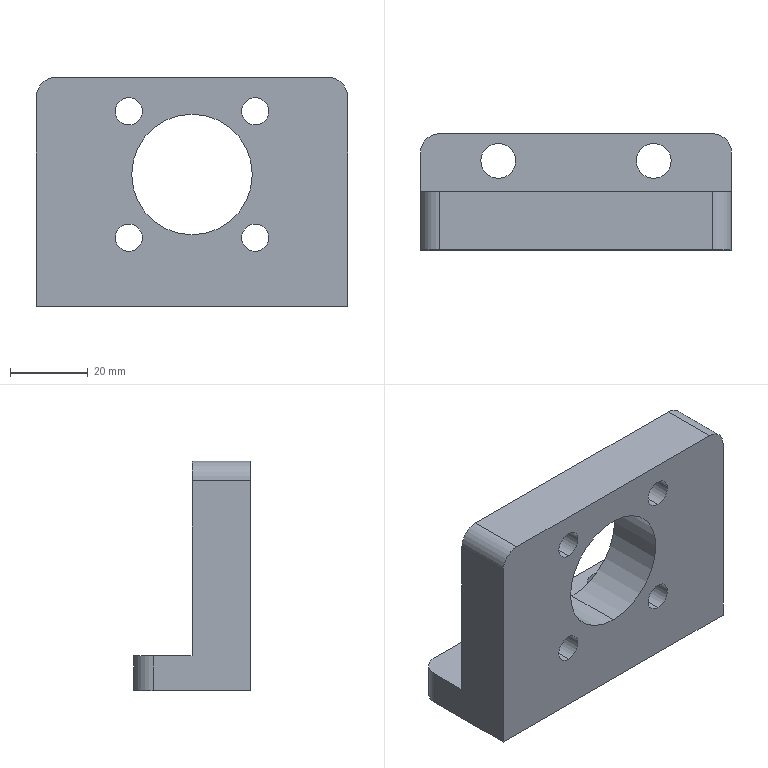Part | 1 solid | 38 faces | box 80 x 30 x 59 mm | volume 65210 mm3 | cylinder 26 | plane 12 | commonest cylinder face diameters 7 x8 11 x8 9 x4 10 x4 31 x2
STEP:
#1=CARTESIAN_POINT('',(16.263,-6.,44.763));
#2=VERTEX_POINT('',#1);
#3=CARTESIAN_POINT('',(16.263,-6.,55.763));
#4=VERTEX_POINT('',#3);
#5=CARTESIAN_POINT('',(16.263,-6.,50.263));
#6=DIRECTION('',(0.,1.,0.));
#7=DIRECTION('',(0.,0.,1.));
#8=AXIS2_PLACEMENT_3D('',#5,#6,#7);
#9=CIRCLE('',#8,5.5);
#10=EDGE_CURVE('',#2,#4,#9,.T.);
#11=ORIENTED_EDGE('',*,*,#10,.F.);
#12=CARTESIAN_POINT('',(16.263,0.,44.763));
#13=VERTEX_POINT('',#12);
#14=CARTESIAN_POINT('',(16.263,0.,44.763));
#15=DIRECTION('',(0.,1.,0.));
#16=VECTOR('',#15,1000.);
#17=LINE('',#14,#16);
#18=EDGE_CURVE('',#2,#13,#17,.T.);
#19=ORIENTED_EDGE('',*,*,#18,.T.);
#20=CARTESIAN_POINT('',(16.263,0.,55.763));
#21=VERTEX_POINT('',#20);
#22=CARTESIAN_POINT('',(16.263,0.,50.263));
#23=DIRECTION('',(0.,1.,0.));
#24=DIRECTION('',(0.,0.,1.));
#25=AXIS2_PLACEMENT_3D('',#22,#23,#24);
#26=CIRCLE('',#25,5.5);
#27=EDGE_CURVE('',#13,#21,#26,.T.);
#28=ORIENTED_EDGE('',*,*,#27,.T.);
#29=CARTESIAN_POINT('',(16.263,0.,55.763));
#30=DIRECTION('',(0.,1.,0.));
#31=VECTOR('',#30,1000.);
#32=LINE('',#29,#31);
#33=EDGE_CURVE('',#4,#21,#32,.T.);
#34=ORIENTED_EDGE('',*,*,#33,.F.);
#35=EDGE_LOOP('',(#11,#19,#28,#34));
#36=FACE_OUTER_BOUND('',#35,.T.);
#37=CARTESIAN_POINT('',(16.263,0.,50.263));
#38=DIRECTION('',(0.,1.,0.));
#39=DIRECTION('',(0.,0.,1.));
#40=AXIS2_PLACEMENT_3D('',#37,#38,#39);
#41=CYLINDRICAL_SURFACE('',#40,5.5);
#42=ADVANCED_FACE('',(#36),#41,.F.);
#43=CARTESIAN_POINT('',(16.263,-15.,46.763));
#44=VERTEX_POINT('',#43);
#45=CARTESIAN_POINT('',(16.263,-15.,53.763));
#46=VERTEX_POINT('',#45);
#47=CARTESIAN_POINT('',(16.263,-15.,50.263));
#48=DIRECTION('',(0.,1.,0.));
#49=DIRECTION('',(0.,0.,1.));
#50=AXIS2_PLACEMENT_3D('',#47,#48,#49);
#51=CIRCLE('',#50,3.5);
#52=EDGE_CURVE('',#44,#46,#51,.T.);
#53=ORIENTED_EDGE('',*,*,#52,.F.);
#54=CARTESIAN_POINT('',(16.263,-6.,46.763));
#55=VERTEX_POINT('',#54);
#56=CARTESIAN_POINT('',(16.263,0.,46.763));
#57=DIRECTION('',(0.,1.,0.));
#58=VECTOR('',#57,1000.);
#59=LINE('',#56,#58);
#60=EDGE_CURVE('',#44,#55,#59,.T.);
#61=ORIENTED_EDGE('',*,*,#60,.T.);
#62=CARTESIAN_POINT('',(16.263,-6.,53.763));
#63=VERTEX_POINT('',#62);
#64=CARTESIAN_POINT('',(16.263,-6.,50.263));
#65=DIRECTION('',(0.,1.,0.));
#66=DIRECTION('',(0.,0.,1.));
#67=AXIS2_PLACEMENT_3D('',#64,#65,#66);
#68=CIRCLE('',#67,3.5);
#69=EDGE_CURVE('',#55,#63,#68,.T.);
#70=ORIENTED_EDGE('',*,*,#69,.T.);
#71=CARTESIAN_POINT('',(16.263,0.,53.763));
#72=DIRECTION('',(0.,1.,0.));
#73=VECTOR('',#72,1000.);
#74=LINE('',#71,#73);
#75=EDGE_CURVE('',#46,#63,#74,.T.);
#76=ORIENTED_EDGE('',*,*,#75,.F.);
#77=EDGE_LOOP('',(#53,#61,#70,#76));
#78=FACE_OUTER_BOUND('',#77,.T.);
#79=CARTESIAN_POINT('',(16.263,0.,50.263));
#80=DIRECTION('',(0.,1.,0.));
#81=DIRECTION('',(0.,0.,1.));
#82=AXIS2_PLACEMENT_3D('',#79,#80,#81);
#83=CYLINDRICAL_SURFACE('',#82,3.5);
#84=ADVANCED_FACE('',(#78),#83,.F.);
#85=CARTESIAN_POINT('',(-16.263,-6.,12.237));
#86=VERTEX_POINT('',#85);
#87=CARTESIAN_POINT('',(-16.263,-6.,23.237));
#88=VERTEX_POINT('',#87);
#89=CARTESIAN_POINT('',(-16.263,-6.,17.737));
#90=DIRECTION('',(0.,1.,0.));
#91=DIRECTION('',(0.,0.,1.));
#92=AXIS2_PLACEMENT_3D('',#89,#90,#91);
#93=CIRCLE('',#92,5.5);
#94=EDGE_CURVE('',#86,#88,#93,.T.);
#95=ORIENTED_EDGE('',*,*,#94,.F.);
#96=CARTESIAN_POINT('',(-16.263,0.,12.237));
#97=VERTEX_POINT('',#96);
#98=CARTESIAN_POINT('',(-16.263,0.,12.237));
#99=DIRECTION('',(0.,1.,0.));
#100=VECTOR('',#99,1000.);
#101=LINE('',#98,#100);
#102=EDGE_CURVE('',#86,#97,#101,.T.);
#103=ORIENTED_EDGE('',*,*,#102,.T.);
#104=CARTESIAN_POINT('',(-16.263,0.,23.237));
#105=VERTEX_POINT('',#104);
#106=CARTESIAN_POINT('',(-16.263,0.,17.737));
#107=DIRECTION('',(0.,1.,0.));
#108=DIRECTION('',(0.,0.,1.));
#109=AXIS2_PLACEMENT_3D('',#106,#107,#108);
#110=CIRCLE('',#109,5.5);
#111=EDGE_CURVE('',#97,#105,#110,.T.);
#112=ORIENTED_EDGE('',*,*,#111,.T.);
#113=CARTESIAN_POINT('',(-16.263,0.,23.237));
#114=DIRECTION('',(0.,1.,0.));
#115=VECTOR('',#114,1000.);
#116=LINE('',#113,#115);
#117=EDGE_CURVE('',#88,#105,#116,.T.);
#118=ORIENTED_EDGE('',*,*,#117,.F.);
#119=EDGE_LOOP('',(#95,#103,#112,#118));
#120=FACE_OUTER_BOUND('',#119,.T.);
#121=CARTESIAN_POINT('',(-16.263,0.,17.737));
#122=DIRECTION('',(0.,1.,0.));
#123=DIRECTION('',(0.,0.,1.));
#124=AXIS2_PLACEMENT_3D('',#121,#122,#123);
#125=CYLINDRICAL_SURFACE('',#124,5.5);
#126=ADVANCED_FACE('',(#120),#125,.F.);
#127=CARTESIAN_POINT('',(-16.263,-15.,14.237));
#128=VERTEX_POINT('',#127);
#129=CARTESIAN_POINT('',(-16.263,-15.,21.237));
#130=VERTEX_POINT('',#129);
#131=CARTESIAN_POINT('',(-16.263,-15.,17.737));
#132=DIRECTION('',(0.,1.,0.));
#133=DIRECTION('',(0.,0.,1.));
#134=AXIS2_PLACEMENT_3D('',#131,#132,#133);
#135=CIRCLE('',#134,3.5);
#136=EDGE_CURVE('',#128,#130,#135,.T.);
#137=ORIENTED_EDGE('',*,*,#136,.F.);
#138=CARTESIAN_POINT('',(-16.263,-6.,14.237));
#139=VERTEX_POINT('',#138);
#140=CARTESIAN_POINT('',(-16.263,0.,14.237));
#141=DIRECTION('',(0.,1.,0.));
#142=VECTOR('',#141,1000.);
#143=LINE('',#140,#142);
#144=EDGE_CURVE('',#128,#139,#143,.T.);
#145=ORIENTED_EDGE('',*,*,#144,.T.);
#146=CARTESIAN_POINT('',(-16.263,-6.,21.237));
#147=VERTEX_POINT('',#146);
#148=CARTESIAN_POINT('',(-16.263,-6.,17.737));
#149=DIRECTION('',(0.,1.,0.));
#150=DIRECTION('',(0.,0.,1.));
#151=AXIS2_PLACEMENT_3D('',#148,#149,#150);
#152=CIRCLE('',#151,3.5);
#153=EDGE_CURVE('',#139,#147,#152,.T.);
#154=ORIENTED_EDGE('',*,*,#153,.T.);
#155=CARTESIAN_POINT('',(-16.263,0.,21.237));
#156=DIRECTION('',(0.,1.,0.));
#157=VECTOR('',#156,1000.);
#158=LINE('',#155,#157);
#159=EDGE_CURVE('',#130,#147,#158,.T.);
#160=ORIENTED_EDGE('',*,*,#159,.F.);
#161=EDGE_LOOP('',(#137,#145,#154,#160));
#162=FACE_OUTER_BOUND('',#161,.T.);
#163=CARTESIAN_POINT('',(-16.263,0.,17.737));
#164=DIRECTION('',(0.,1.,0.));
#165=DIRECTION('',(0.,0.,1.));
#166=AXIS2_PLACEMENT_3D('',#163,#164,#165);
#167=CYLINDRICAL_SURFACE('',#166,3.5);
#168=ADVANCED_FACE('',(#162),#167,.F.);
#169=CARTESIAN_POINT('',(-16.263,-6.,44.763));
#170=VERTEX_POINT('',#169);
#171=CARTESIAN_POINT('',(-16.263,-6.,55.763));
#172=VERTEX_POINT('',#171);
#173=CARTESIAN_POINT('',(-16.263,-6.,50.263));
#174=DIRECTION('',(0.,1.,0.));
#175=DIRECTION('',(0.,0.,1.));
#176=AXIS2_PLACEMENT_3D('',#173,#174,#175);
#177=CIRCLE('',#176,5.5);
#178=EDGE_CURVE('',#170,#172,#177,.T.);
#179=ORIENTED_EDGE('',*,*,#178,.F.);
#180=CARTESIAN_POINT('',(-16.263,0.,44.763));
#181=VERTEX_POINT('',#180);
#182=CARTESIAN_POINT('',(-16.263,0.,44.763));
#183=DIRECTION('',(0.,1.,0.));
#184=VECTOR('',#183,1000.);
#185=LINE('',#182,#184);
#186=EDGE_CURVE('',#170,#181,#185,.T.);
#187=ORIENTED_EDGE('',*,*,#186,.T.);
#188=CARTESIAN_POINT('',(-16.263,0.,55.763));
#189=VERTEX_POINT('',#188);
#190=CARTESIAN_POINT('',(-16.263,0.,50.263));
#191=DIRECTION('',(0.,1.,0.));
#192=DIRECTION('',(0.,0.,1.));
#193=AXIS2_PLACEMENT_3D('',#190,#191,#192);
#194=CIRCLE('',#193,5.5);
#195=EDGE_CURVE('',#181,#189,#194,.T.);
#196=ORIENTED_EDGE('',*,*,#195,.T.);
#197=CARTESIAN_POINT('',(-16.263,0.,55.763));
#198=DIRECTION('',(0.,1.,0.));
#199=VECTOR('',#198,1000.);
#200=LINE('',#197,#199);
#201=EDGE_CURVE('',#172,#189,#200,.T.);
#202=ORIENTED_EDGE('',*,*,#201,.F.);
#203=EDGE_LOOP('',(#179,#187,#196,#202));
#204=FACE_OUTER_BOUND('',#203,.T.);
#205=CARTESIAN_POINT('',(-16.263,0.,50.263));
#206=DIRECTION('',(0.,1.,0.));
#207=DIRECTION('',(0.,0.,1.));
#208=AXIS2_PLACEMENT_3D('',#205,#206,#207);
#209=CYLINDRICAL_SURFACE('',#208,5.5);
#210=ADVANCED_FACE('',(#204),#209,.F.);
#211=CARTESIAN_POINT('',(-16.263,-15.,46.763));
#212=VERTEX_POINT('',#211);
#213=CARTESIAN_POINT('',(-16.263,-15.,53.763));
#214=VERTEX_POINT('',#213);
#215=CARTESIAN_POINT('',(-16.263,-15.,50.263));
#216=DIRECTION('',(0.,1.,0.));
#217=DIRECTION('',(0.,0.,1.));
#218=AXIS2_PLACEMENT_3D('',#215,#216,#217);
#219=CIRCLE('',#218,3.5);
#220=EDGE_CURVE('',#212,#214,#219,.T.);
#221=ORIENTED_EDGE('',*,*,#220,.F.);
#222=CARTESIAN_POINT('',(-16.263,-6.,46.763));
#223=VERTEX_POINT('',#222);
#224=CARTESIAN_POINT('',(-16.263,0.,46.763));
#225=DIRECTION('',(0.,1.,0.));
#226=VECTOR('',#225,1000.);
#227=LINE('',#224,#226);
#228=EDGE_CURVE('',#212,#223,#227,.T.);
#229=ORIENTED_EDGE('',*,*,#228,.T.);
#230=CARTESIAN_POINT('',(-16.263,-6.,53.763));
#231=VERTEX_POINT('',#230);
#232=CARTESIAN_POINT('',(-16.263,-6.,50.263));
#233=DIRECTION('',(0.,1.,0.));
#234=DIRECTION('',(0.,0.,1.));
#235=AXIS2_PLACEMENT_3D('',#232,#233,#234);
#236=CIRCLE('',#235,3.5);
#237=EDGE_CURVE('',#223,#231,#236,.T.);
#238=ORIENTED_EDGE('',*,*,#237,.T.);
#239=CARTESIAN_POINT('',(-16.263,0.,53.763));
#240=DIRECTION('',(0.,1.,0.));
#241=VECTOR('',#240,1000.);
#242=LINE('',#239,#241);
#243=EDGE_CURVE('',#214,#231,#242,.T.);
#244=ORIENTED_EDGE('',*,*,#243,.F.);
#245=EDGE_LOOP('',(#221,#229,#238,#244));
#246=FACE_OUTER_BOUND('',#245,.T.);
#247=CARTESIAN_POINT('',(-16.263,0.,50.263));
#248=DIRECTION('',(0.,1.,0.));
#249=DIRECTION('',(0.,0.,1.));
#250=AXIS2_PLACEMENT_3D('',#247,#248,#249);
#251=CYLINDRICAL_SURFACE('',#250,3.5);
#252=ADVANCED_FACE('',(#246),#251,.F.);
#253=CARTESIAN_POINT('',(16.263,-6.,12.237));
#254=VERTEX_POINT('',#253);
#255=CARTESIAN_POINT('',(16.263,-6.,23.237));
#256=VERTEX_POINT('',#255);
#257=CARTESIAN_POINT('',(16.263,-6.,17.737));
#258=DIRECTION('',(0.,1.,0.));
#259=DIRECTION('',(0.,0.,1.));
#260=AXIS2_PLACEMENT_3D('',#257,#258,#259);
#261=CIRCLE('',#260,5.5);
#262=EDGE_CURVE('',#254,#256,#261,.T.);
#263=ORIENTED_EDGE('',*,*,#262,.F.);
#264=CARTESIAN_POINT('',(16.263,0.,12.237));
#265=VERTEX_POINT('',#264);
#266=CARTESIAN_POINT('',(16.263,0.,12.237));
#267=DIRECTION('',(0.,1.,0.));
#268=VECTOR('',#267,1000.);
#269=LINE('',#266,#268);
#270=EDGE_CURVE('',#254,#265,#269,.T.);
#271=ORIENTED_EDGE('',*,*,#270,.T.);
#272=CARTESIAN_POINT('',(16.263,0.,23.237));
#273=VERTEX_POINT('',#272);
#274=CARTESIAN_POINT('',(16.263,0.,17.737));
#275=DIRECTION('',(0.,1.,0.));
#276=DIRECTION('',(0.,0.,1.));
#277=AXIS2_PLACEMENT_3D('',#274,#275,#276);
#278=CIRCLE('',#277,5.5);
#279=EDGE_CURVE('',#265,#273,#278,.T.);
#280=ORIENTED_EDGE('',*,*,#279,.T.);
#281=CARTESIAN_POINT('',(16.263,0.,23.237));
#282=DIRECTION('',(0.,1.,0.));
#283=VECTOR('',#282,1000.);
#284=LINE('',#281,#283);
#285=EDGE_CURVE('',#256,#273,#284,.T.);
#286=ORIENTED_EDGE('',*,*,#285,.F.);
#287=EDGE_LOOP('',(#263,#271,#280,#286));
#288=FACE_OUTER_BOUND('',#287,.T.);
#289=CARTESIAN_POINT('',(16.263,0.,17.737));
#290=DIRECTION('',(0.,1.,0.));
#291=DIRECTION('',(0.,0.,1.));
#292=AXIS2_PLACEMENT_3D('',#289,#290,#291);
#293=CYLINDRICAL_SURFACE('',#292,5.5);
#294=ADVANCED_FACE('',(#288),#293,.F.);
#295=CARTESIAN_POINT('',(16.263,-15.,14.237));
#296=VERTEX_POINT('',#295);
#297=CARTESIAN_POINT('',(16.263,-15.,21.237));
#298=VERTEX_POINT('',#297);
#299=CARTESIAN_POINT('',(16.263,-15.,17.737));
#300=DIRECTION('',(0.,1.,0.));
#301=DIRECTION('',(0.,0.,1.));
#302=AXIS2_PLACEMENT_3D('',#299,#300,#301);
#303=CIRCLE('',#302,3.5);
#304=EDGE_CURVE('',#296,#298,#303,.T.);
#305=ORIENTED_EDGE('',*,*,#304,.F.);
#306=CARTESIAN_POINT('',(16.263,-6.,14.237));
#307=VERTEX_POINT('',#306);
#308=CARTESIAN_POINT('',(16.263,0.,14.237));
#309=DIRECTION('',(0.,1.,0.));
#310=VECTOR('',#309,1000.);
#311=LINE('',#308,#310);
#312=EDGE_CURVE('',#296,#307,#311,.T.);
#313=ORIENTED_EDGE('',*,*,#312,.T.);
#314=CARTESIAN_POINT('',(16.263,-6.,21.237));
#315=VERTEX_POINT('',#314);
#316=CARTESIAN_POINT('',(16.263,-6.,17.737));
#317=DIRECTION('',(0.,1.,0.));
#318=DIRECTION('',(0.,0.,1.));
#319=AXIS2_PLACEMENT_3D('',#316,#317,#318);
#320=CIRCLE('',#319,3.5);
#321=EDGE_CURVE('',#307,#315,#320,.T.);
#322=ORIENTED_EDGE('',*,*,#321,.T.);
#323=CARTESIAN_POINT('',(16.263,0.,21.237));
#324=DIRECTION('',(0.,1.,0.));
#325=VECTOR('',#324,1000.);
#326=LINE('',#323,#325);
#327=EDGE_CURVE('',#298,#315,#326,.T.);
#328=ORIENTED_EDGE('',*,*,#327,.F.);
#329=EDGE_LOOP('',(#305,#313,#322,#328));
#330=FACE_OUTER_BOUND('',#329,.T.);
#331=CARTESIAN_POINT('',(16.263,0.,17.737));
#332=DIRECTION('',(0.,1.,0.));
#333=DIRECTION('',(0.,0.,1.));
#334=AXIS2_PLACEMENT_3D('',#331,#332,#333);
#335=CYLINDRICAL_SURFACE('',#334,3.5);
#336=ADVANCED_FACE('',(#330),#335,.F.);
#337=CARTESIAN_POINT('',(0.,0.,49.5));
#338=VERTEX_POINT('',#337);
#339=CARTESIAN_POINT('',(0.,0.,18.5));
#340=VERTEX_POINT('',#339);
#341=CARTESIAN_POINT('',(0.,0.,34.));
#342=DIRECTION('',(0.,-1.,0.));
#343=DIRECTION('',(0.,0.,-1.));
#344=AXIS2_PLACEMENT_3D('',#341,#342,#343);
#345=CIRCLE('',#344,15.5);
#346=EDGE_CURVE('',#338,#340,#345,.T.);
#347=ORIENTED_EDGE('',*,*,#346,.F.);
#348=CARTESIAN_POINT('',(0.,-15.,49.5));
#349=VERTEX_POINT('',#348);
#350=CARTESIAN_POINT('',(0.,-15.,49.5));
#351=DIRECTION('',(0.,-1.,0.));
#352=VECTOR('',#351,1000.);
#353=LINE('',#350,#352);
#354=EDGE_CURVE('',#338,#349,#353,.T.);
#355=ORIENTED_EDGE('',*,*,#354,.T.);
#356=CARTESIAN_POINT('',(0.,-15.,18.5));
#357=VERTEX_POINT('',#356);
#358=CARTESIAN_POINT('',(0.,-15.,34.));
#359=DIRECTION('',(0.,-1.,0.));
#360=DIRECTION('',(0.,0.,-1.));
#361=AXIS2_PLACEMENT_3D('',#358,#359,#360);
#362=CIRCLE('',#361,15.5);
#363=EDGE_CURVE('',#349,#357,#362,.T.);
#364=ORIENTED_EDGE('',*,*,#363,.T.);
#365=CARTESIAN_POINT('',(0.,-15.,18.5));
#366=DIRECTION('',(0.,-1.,0.));
#367=VECTOR('',#366,1000.);
#368=LINE('',#365,#367);
#369=EDGE_CURVE('',#340,#357,#368,.T.);
#370=ORIENTED_EDGE('',*,*,#369,.F.);
#371=EDGE_LOOP('',(#347,#355,#364,#370));
#372=FACE_OUTER_BOUND('',#371,.T.);
#373=CARTESIAN_POINT('',(0.,-15.,34.));
#374=DIRECTION('',(0.,-1.,0.));
#375=DIRECTION('',(0.,0.,-1.));
#376=AXIS2_PLACEMENT_3D('',#373,#374,#375);
#377=CYLINDRICAL_SURFACE('',#376,15.5);
#378=ADVANCED_FACE('',(#372),#377,.F.);
#379=CARTESIAN_POINT('',(15.5,8.,0.));
#380=VERTEX_POINT('',#379);
#381=CARTESIAN_POINT('',(24.5,8.,0.));
#382=VERTEX_POINT('',#381);
#383=CARTESIAN_POINT('',(20.,8.,0.));
#384=DIRECTION('',(0.,0.,1.));
#385=DIRECTION('',(1.,0.,0.));
#386=AXIS2_PLACEMENT_3D('',#383,#384,#385);
#387=CIRCLE('',#386,4.5);
#388=EDGE_CURVE('',#380,#382,#387,.T.);
#389=ORIENTED_EDGE('',*,*,#388,.F.);
#390=CARTESIAN_POINT('',(15.5,8.,9.));
#391=VERTEX_POINT('',#390);
#392=CARTESIAN_POINT('',(15.5,8.,9.));
#393=DIRECTION('',(0.,0.,1.));
#394=VECTOR('',#393,1000.);
#395=LINE('',#392,#394);
#396=EDGE_CURVE('',#380,#391,#395,.T.);
#397=ORIENTED_EDGE('',*,*,#396,.T.);
#398=CARTESIAN_POINT('',(24.5,8.,9.));
#399=VERTEX_POINT('',#398);
#400=CARTESIAN_POINT('',(20.,8.,9.));
#401=DIRECTION('',(0.,0.,1.));
#402=DIRECTION('',(1.,0.,0.));
#403=AXIS2_PLACEMENT_3D('',#400,#401,#402);
#404=CIRCLE('',#403,4.5);
#405=EDGE_CURVE('',#391,#399,#404,.T.);
#406=ORIENTED_EDGE('',*,*,#405,.T.);
#407=CARTESIAN_POINT('',(24.5,8.,9.));
#408=DIRECTION('',(0.,0.,1.));
#409=VECTOR('',#408,1000.);
#410=LINE('',#407,#409);
#411=EDGE_CURVE('',#382,#399,#410,.T.);
#412=ORIENTED_EDGE('',*,*,#411,.F.);
#413=EDGE_LOOP('',(#389,#397,#406,#412));
#414=FACE_OUTER_BOUND('',#413,.T.);
#415=CARTESIAN_POINT('',(20.,8.,9.));
#416=DIRECTION('',(0.,0.,1.));
#417=DIRECTION('',(1.,0.,0.));
#418=AXIS2_PLACEMENT_3D('',#415,#416,#417);
#419=CYLINDRICAL_SURFACE('',#418,4.5);
#420=ADVANCED_FACE('',(#414),#419,.F.);
#421=CARTESIAN_POINT('',(-24.5,8.,0.));
#422=VERTEX_POINT('',#421);
#423=CARTESIAN_POINT('',(-15.5,8.,0.));
#424=VERTEX_POINT('',#423);
#425=CARTESIAN_POINT('',(-20.,8.,0.));
#426=DIRECTION('',(0.,0.,1.));
#427=DIRECTION('',(1.,0.,0.));
#428=AXIS2_PLACEMENT_3D('',#425,#426,#427);
#429=CIRCLE('',#428,4.5);
#430=EDGE_CURVE('',#422,#424,#429,.T.);
#431=ORIENTED_EDGE('',*,*,#430,.F.);
#432=CARTESIAN_POINT('',(-24.5,8.,9.));
#433=VERTEX_POINT('',#432);
#434=CARTESIAN_POINT('',(-24.5,8.,9.));
#435=DIRECTION('',(0.,0.,1.));
#436=VECTOR('',#435,1000.);
#437=LINE('',#434,#436);
#438=EDGE_CURVE('',#422,#433,#437,.T.);
#439=ORIENTED_EDGE('',*,*,#438,.T.);
#440=CARTESIAN_POINT('',(-15.5,8.,9.));
#441=VERTEX_POINT('',#440);
#442=CARTESIAN_POINT('',(-20.,8.,9.));
#443=DIRECTION('',(0.,0.,1.));
#444=DIRECTION('',(1.,0.,0.));
#445=AXIS2_PLACEMENT_3D('',#442,#443,#444);
#446=CIRCLE('',#445,4.5);
#447=EDGE_CURVE('',#433,#441,#446,.T.);
#448=ORIENTED_EDGE('',*,*,#447,.T.);
#449=CARTESIAN_POINT('',(-15.5,8.,9.));
#450=DIRECTION('',(0.,0.,1.));
#451=VECTOR('',#450,1000.);
#452=LINE('',#449,#451);
#453=EDGE_CURVE('',#424,#441,#452,.T.);
#454=ORIENTED_EDGE('',*,*,#453,.F.);
#455=EDGE_LOOP('',(#431,#439,#448,#454));
#456=FACE_OUTER_BOUND('',#455,.T.);
#457=CARTESIAN_POINT('',(-20.,8.,9.));
#458=DIRECTION('',(0.,0.,1.));
#459=DIRECTION('',(1.,0.,0.));
#460=AXIS2_PLACEMENT_3D('',#457,#458,#459);
#461=CYLINDRICAL_SURFACE('',#460,4.5);
#462=ADVANCED_FACE('',(#456),#461,.F.);
#463=CARTESIAN_POINT('',(-35.,-15.,59.));
#464=VERTEX_POINT('',#463);
#465=CARTESIAN_POINT('',(-40.,-15.,54.));
#466=VERTEX_POINT('',#465);
#467=CARTESIAN_POINT('',(-35.,-15.,54.));
#468=DIRECTION('',(0.,-1.,0.));
#469=DIRECTION('',(0.,0.,-1.));
#470=AXIS2_PLACEMENT_3D('',#467,#468,#469);
#471=CIRCLE('',#470,5.);
#472=EDGE_CURVE('',#464,#466,#471,.T.);
#473=ORIENTED_EDGE('',*,*,#472,.F.);
#474=CARTESIAN_POINT('',(-35.,0.,59.));
#475=VERTEX_POINT('',#474);
#476=CARTESIAN_POINT('',(-35.,0.,59.));
#477=DIRECTION('',(0.,-1.,0.));
#478=VECTOR('',#477,1000.);
#479=LINE('',#476,#478);
#480=EDGE_CURVE('',#475,#464,#479,.T.);
#481=ORIENTED_EDGE('',*,*,#480,.F.);
#482=CARTESIAN_POINT('',(-40.,0.,54.));
#483=VERTEX_POINT('',#482);
#484=CARTESIAN_POINT('',(-35.,0.,54.));
#485=DIRECTION('',(0.,-1.,0.));
#486=DIRECTION('',(0.,0.,-1.));
#487=AXIS2_PLACEMENT_3D('',#484,#485,#486);
#488=CIRCLE('',#487,5.);
#489=EDGE_CURVE('',#475,#483,#488,.T.);
#490=ORIENTED_EDGE('',*,*,#489,.T.);
#491=CARTESIAN_POINT('',(-40.,0.,54.));
#492=DIRECTION('',(0.,-1.,0.));
#493=VECTOR('',#492,1000.);
#494=LINE('',#491,#493);
#495=EDGE_CURVE('',#483,#466,#494,.T.);
#496=ORIENTED_EDGE('',*,*,#495,.T.);
#497=EDGE_LOOP('',(#473,#481,#490,#496));
#498=FACE_OUTER_BOUND('',#497,.T.);
#499=CARTESIAN_POINT('',(-35.,0.,54.));
#500=DIRECTION('',(0.,-1.,0.));
#501=DIRECTION('',(0.,0.,-1.));
#502=AXIS2_PLACEMENT_3D('',#499,#500,#501);
#503=CYLINDRICAL_SURFACE('',#502,5.);
#504=ADVANCED_FACE('',(#498),#503,.T.);
#505=CARTESIAN_POINT('',(35.,-15.,59.));
#506=VERTEX_POINT('',#505);
#507=CARTESIAN_POINT('',(35.,-15.,59.));
#508=DIRECTION('',(-1.,0.,0.));
#509=VECTOR('',#508,1000.);
#510=LINE('',#507,#509);
#511=EDGE_CURVE('',#506,#464,#510,.T.);
#512=ORIENTED_EDGE('',*,*,#511,.F.);
#513=CARTESIAN_POINT('',(35.,0.,59.));
#514=VERTEX_POINT('',#513);
#515=CARTESIAN_POINT('',(35.,0.,59.));
#516=DIRECTION('',(0.,-1.,0.));
#517=VECTOR('',#516,1000.);
#518=LINE('',#515,#517);
#519=EDGE_CURVE('',#514,#506,#518,.T.);
#520=ORIENTED_EDGE('',*,*,#519,.F.);
#521=CARTESIAN_POINT('',(35.,0.,59.));
#522=DIRECTION('',(-1.,0.,0.));
#523=VECTOR('',#522,1000.);
#524=LINE('',#521,#523);
#525=EDGE_CURVE('',#514,#475,#524,.T.);
#526=ORIENTED_EDGE('',*,*,#525,.T.);
#527=ORIENTED_EDGE('',*,*,#480,.T.);
#528=EDGE_LOOP('',(#512,#520,#526,#527));
#529=FACE_OUTER_BOUND('',#528,.T.);
#530=CARTESIAN_POINT('',(35.,0.,59.));
#531=DIRECTION('',(0.,0.,1.));
#532=DIRECTION('',(1.,0.,0.));
#533=AXIS2_PLACEMENT_3D('',#530,#531,#532);
#534=PLANE('',#533);
#535=ADVANCED_FACE('',(#529),#534,.T.);
#536=CARTESIAN_POINT('',(40.,-15.,54.));
#537=VERTEX_POINT('',#536);
#538=CARTESIAN_POINT('',(35.,-15.,54.));
#539=DIRECTION('',(0.,-1.,0.));
#540=DIRECTION('',(0.,0.,-1.));
#541=AXIS2_PLACEMENT_3D('',#538,#539,#540);
#542=CIRCLE('',#541,5.);
#543=EDGE_CURVE('',#537,#506,#542,.T.);
#544=ORIENTED_EDGE('',*,*,#543,.F.);
#545=CARTESIAN_POINT('',(40.,0.,54.));
#546=VERTEX_POINT('',#545);
#547=CARTESIAN_POINT('',(40.,0.,54.));
#548=DIRECTION('',(0.,-1.,0.));
#549=VECTOR('',#548,1000.);
#550=LINE('',#547,#549);
#551=EDGE_CURVE('',#546,#537,#550,.T.);
#552=ORIENTED_EDGE('',*,*,#551,.F.);
#553=CARTESIAN_POINT('',(35.,0.,54.));
#554=DIRECTION('',(0.,-1.,0.));
#555=DIRECTION('',(0.,0.,-1.));
#556=AXIS2_PLACEMENT_3D('',#553,#554,#555);
#557=CIRCLE('',#556,5.);
#558=EDGE_CURVE('',#546,#514,#557,.T.);
#559=ORIENTED_EDGE('',*,*,#558,.T.);
#560=ORIENTED_EDGE('',*,*,#519,.T.);
#561=EDGE_LOOP('',(#544,#552,#559,#560));
#562=FACE_OUTER_BOUND('',#561,.T.);
#563=CARTESIAN_POINT('',(35.,0.,54.));
#564=DIRECTION('',(0.,-1.,0.));
#565=DIRECTION('',(0.,0.,-1.));
#566=AXIS2_PLACEMENT_3D('',#563,#564,#565);
#567=CYLINDRICAL_SURFACE('',#566,5.);
#568=ADVANCED_FACE('',(#562),#567,.T.);
#569=CARTESIAN_POINT('',(16.263,0.,50.263));
#570=DIRECTION('',(0.,1.,0.));
#571=DIRECTION('',(0.,0.,1.));
#572=AXIS2_PLACEMENT_3D('',#569,#570,#571);
#573=CIRCLE('',#572,5.5);
#574=EDGE_CURVE('',#21,#13,#573,.T.);
#575=ORIENTED_EDGE('',*,*,#574,.F.);
#576=ORIENTED_EDGE('',*,*,#27,.F.);
#577=EDGE_LOOP('',(#575,#576));
#578=FACE_BOUND('',#577,.T.);
#579=CARTESIAN_POINT('',(-16.263,0.,17.737));
#580=DIRECTION('',(0.,1.,0.));
#581=DIRECTION('',(0.,0.,1.));
#582=AXIS2_PLACEMENT_3D('',#579,#580,#581);
#583=CIRCLE('',#582,5.5);
#584=EDGE_CURVE('',#105,#97,#583,.T.);
#585=ORIENTED_EDGE('',*,*,#584,.F.);
#586=ORIENTED_EDGE('',*,*,#111,.F.);
#587=EDGE_LOOP('',(#585,#586));
#588=FACE_BOUND('',#587,.T.);
#589=CARTESIAN_POINT('',(-16.263,0.,50.263));
#590=DIRECTION('',(0.,1.,0.));
#591=DIRECTION('',(0.,0.,1.));
#592=AXIS2_PLACEMENT_3D('',#589,#590,#591);
#593=CIRCLE('',#592,5.5);
#594=EDGE_CURVE('',#189,#181,#593,.T.);
#595=ORIENTED_EDGE('',*,*,#594,.F.);
#596=ORIENTED_EDGE('',*,*,#195,.F.);
#597=EDGE_LOOP('',(#595,#596));
#598=FACE_BOUND('',#597,.T.);
#599=CARTESIAN_POINT('',(16.263,0.,17.737));
#600=DIRECTION('',(0.,1.,0.));
#601=DIRECTION('',(0.,0.,1.));
#602=AXIS2_PLACEMENT_3D('',#599,#600,#601);
#603=CIRCLE('',#602,5.5);
#604=EDGE_CURVE('',#273,#265,#603,.T.);
#605=ORIENTED_EDGE('',*,*,#604,.F.);
#606=ORIENTED_EDGE('',*,*,#279,.F.);
#607=EDGE_LOOP('',(#605,#606));
#608=FACE_BOUND('',#607,.T.);
#609=CARTESIAN_POINT('',(0.,0.,34.));
#610=DIRECTION('',(0.,-1.,0.));
#611=DIRECTION('',(0.,0.,-1.));
#612=AXIS2_PLACEMENT_3D('',#609,#610,#611);
#613=CIRCLE('',#612,15.5);
#614=EDGE_CURVE('',#340,#338,#613,.T.);
#615=ORIENTED_EDGE('',*,*,#614,.T.);
#616=ORIENTED_EDGE('',*,*,#346,.T.);
#617=EDGE_LOOP('',(#615,#616));
#618=FACE_BOUND('',#617,.T.);
#619=ORIENTED_EDGE('',*,*,#489,.F.);
#620=ORIENTED_EDGE('',*,*,#525,.F.);
#621=ORIENTED_EDGE('',*,*,#558,.F.);
#622=CARTESIAN_POINT('',(40.,0.,9.));
#623=VERTEX_POINT('',#622);
#624=CARTESIAN_POINT('',(40.,0.,9.));
#625=DIRECTION('',(0.,0.,1.));
#626=VECTOR('',#625,1000.);
#627=LINE('',#624,#626);
#628=EDGE_CURVE('',#623,#546,#627,.T.);
#629=ORIENTED_EDGE('',*,*,#628,.F.);
#630=CARTESIAN_POINT('',(-40.,0.,9.));
#631=VERTEX_POINT('',#630);
#632=CARTESIAN_POINT('',(40.,0.,9.));
#633=DIRECTION('',(1.,0.,0.));
#634=VECTOR('',#633,1000.);
#635=LINE('',#632,#634);
#636=EDGE_CURVE('',#631,#623,#635,.T.);
#637=ORIENTED_EDGE('',*,*,#636,.F.);
#638=CARTESIAN_POINT('',(-40.,0.,9.));
#639=DIRECTION('',(0.,0.,1.));
#640=VECTOR('',#639,1000.);
#641=LINE('',#638,#640);
#642=EDGE_CURVE('',#631,#483,#641,.T.);
#643=ORIENTED_EDGE('',*,*,#642,.T.);
#644=EDGE_LOOP('',(#619,#620,#621,#629,#637,#643));
#645=FACE_OUTER_BOUND('',#644,.T.);
#646=CARTESIAN_POINT('',(-35.,0.,54.));
#647=DIRECTION('',(0.,-1.,0.));
#648=DIRECTION('',(0.,0.,-1.));
#649=AXIS2_PLACEMENT_3D('',#646,#647,#648);
#650=PLANE('',#649);
#651=ADVANCED_FACE('',(#578,#588,#598,#608,#618,#645),#650,.F.);
#652=CARTESIAN_POINT('',(16.263,-15.,50.263));
#653=DIRECTION('',(0.,1.,0.));
#654=DIRECTION('',(0.,0.,1.));
#655=AXIS2_PLACEMENT_3D('',#652,#653,#654);
#656=CIRCLE('',#655,3.5);
#657=EDGE_CURVE('',#46,#44,#656,.T.);
#658=ORIENTED_EDGE('',*,*,#657,.T.);
#659=ORIENTED_EDGE('',*,*,#52,.T.);
#660=EDGE_LOOP('',(#658,#659));
#661=FACE_BOUND('',#660,.T.);
#662=CARTESIAN_POINT('',(-16.263,-15.,17.737));
#663=DIRECTION('',(0.,1.,0.));
#664=DIRECTION('',(0.,0.,1.));
#665=AXIS2_PLACEMENT_3D('',#662,#663,#664);
#666=CIRCLE('',#665,3.5);
#667=EDGE_CURVE('',#130,#128,#666,.T.);
#668=ORIENTED_EDGE('',*,*,#667,.T.);
#669=ORIENTED_EDGE('',*,*,#136,.T.);
#670=EDGE_LOOP('',(#668,#669));
#671=FACE_BOUND('',#670,.T.);
#672=CARTESIAN_POINT('',(-16.263,-15.,50.263));
#673=DIRECTION('',(0.,1.,0.));
#674=DIRECTION('',(0.,0.,1.));
#675=AXIS2_PLACEMENT_3D('',#672,#673,#674);
#676=CIRCLE('',#675,3.5);
#677=EDGE_CURVE('',#214,#212,#676,.T.);
#678=ORIENTED_EDGE('',*,*,#677,.T.);
#679=ORIENTED_EDGE('',*,*,#220,.T.);
#680=EDGE_LOOP('',(#678,#679));
#681=FACE_BOUND('',#680,.T.);
#682=CARTESIAN_POINT('',(16.263,-15.,17.737));
#683=DIRECTION('',(0.,1.,0.));
#684=DIRECTION('',(0.,0.,1.));
#685=AXIS2_PLACEMENT_3D('',#682,#683,#684);
#686=CIRCLE('',#685,3.5);
#687=EDGE_CURVE('',#298,#296,#686,.T.);
#688=ORIENTED_EDGE('',*,*,#687,.T.);
#689=ORIENTED_EDGE('',*,*,#304,.T.);
#690=EDGE_LOOP('',(#688,#689));
#691=FACE_BOUND('',#690,.T.);
#692=CARTESIAN_POINT('',(0.,-15.,34.));
#693=DIRECTION('',(0.,-1.,0.));
#694=DIRECTION('',(0.,0.,-1.));
#695=AXIS2_PLACEMENT_3D('',#692,#693,#694);
#696=CIRCLE('',#695,15.5);
#697=EDGE_CURVE('',#357,#349,#696,.T.);
#698=ORIENTED_EDGE('',*,*,#697,.F.);
#699=ORIENTED_EDGE('',*,*,#363,.F.);
#700=EDGE_LOOP('',(#698,#699));
#701=FACE_BOUND('',#700,.T.);
#702=ORIENTED_EDGE('',*,*,#472,.T.);
#703=CARTESIAN_POINT('',(-40.,-15.,0.));
#704=VERTEX_POINT('',#703);
#705=CARTESIAN_POINT('',(-40.,-15.,9.));
#706=DIRECTION('',(0.,0.,1.));
#707=VECTOR('',#706,1000.);
#708=LINE('',#705,#707);
#709=EDGE_CURVE('',#704,#466,#708,.T.);
#710=ORIENTED_EDGE('',*,*,#709,.F.);
#711=CARTESIAN_POINT('',(40.,-15.,0.));
#712=VERTEX_POINT('',#711);
#713=CARTESIAN_POINT('',(-40.,-15.,0.));
#714=DIRECTION('',(-1.,0.,0.));
#715=VECTOR('',#714,1000.);
#716=LINE('',#713,#715);
#717=EDGE_CURVE('',#712,#704,#716,.T.);
#718=ORIENTED_EDGE('',*,*,#717,.F.);
#719=CARTESIAN_POINT('',(40.,-15.,9.));
#720=DIRECTION('',(0.,0.,1.));
#721=VECTOR('',#720,1000.);
#722=LINE('',#719,#721);
#723=EDGE_CURVE('',#712,#537,#722,.T.);
#724=ORIENTED_EDGE('',*,*,#723,.T.);
#725=ORIENTED_EDGE('',*,*,#543,.T.);
#726=ORIENTED_EDGE('',*,*,#511,.T.);
#727=EDGE_LOOP('',(#702,#710,#718,#724,#725,#726));
#728=FACE_OUTER_BOUND('',#727,.T.);
#729=CARTESIAN_POINT('',(-35.,-15.,54.));
#730=DIRECTION('',(0.,-1.,0.));
#731=DIRECTION('',(0.,0.,-1.));
#732=AXIS2_PLACEMENT_3D('',#729,#730,#731);
#733=PLANE('',#732);
#734=ADVANCED_FACE('',(#661,#671,#681,#691,#701,#728),#733,.T.);
#735=ORIENTED_EDGE('',*,*,#551,.T.);
#736=ORIENTED_EDGE('',*,*,#723,.F.);
#737=CARTESIAN_POINT('',(40.,10.,0.));
#738=VERTEX_POINT('',#737);
#739=CARTESIAN_POINT('',(40.,-15.,0.));
#740=DIRECTION('',(0.,-1.,0.));
#741=VECTOR('',#740,1000.);
#742=LINE('',#739,#741);
#743=EDGE_CURVE('',#738,#712,#742,.T.);
#744=ORIENTED_EDGE('',*,*,#743,.F.);
#745=CARTESIAN_POINT('',(40.,10.,9.));
#746=VERTEX_POINT('',#745);
#747=CARTESIAN_POINT('',(40.,10.,0.));
#748=DIRECTION('',(0.,0.,1.));
#749=VECTOR('',#748,1000.);
#750=LINE('',#747,#749);
#751=EDGE_CURVE('',#738,#746,#750,.T.);
#752=ORIENTED_EDGE('',*,*,#751,.T.);
#753=CARTESIAN_POINT('',(40.,-15.,9.));
#754=DIRECTION('',(0.,-1.,0.));
#755=VECTOR('',#754,1000.);
#756=LINE('',#753,#755);
#757=EDGE_CURVE('',#746,#623,#756,.T.);
#758=ORIENTED_EDGE('',*,*,#757,.T.);
#759=ORIENTED_EDGE('',*,*,#628,.T.);
#760=EDGE_LOOP('',(#735,#736,#744,#752,#758,#759));
#761=FACE_OUTER_BOUND('',#760,.T.);
#762=CARTESIAN_POINT('',(40.,-15.,9.));
#763=DIRECTION('',(-1.,0.,0.));
#764=DIRECTION('',(0.,0.,1.));
#765=AXIS2_PLACEMENT_3D('',#762,#763,#764);
#766=PLANE('',#765);
#767=ADVANCED_FACE('',(#761),#766,.F.);
#768=ORIENTED_EDGE('',*,*,#495,.F.);
#769=ORIENTED_EDGE('',*,*,#642,.F.);
#770=CARTESIAN_POINT('',(-40.,10.,9.));
#771=VERTEX_POINT('',#770);
#772=CARTESIAN_POINT('',(-40.,10.,9.));
#773=DIRECTION('',(0.,1.,0.));
#774=VECTOR('',#773,1000.);
#775=LINE('',#772,#774);
#776=EDGE_CURVE('',#631,#771,#775,.T.);
#777=ORIENTED_EDGE('',*,*,#776,.T.);
#778=CARTESIAN_POINT('',(-40.,10.,0.));
#779=VERTEX_POINT('',#778);
#780=CARTESIAN_POINT('',(-40.,10.,0.));
#781=DIRECTION('',(0.,0.,1.));
#782=VECTOR('',#781,1000.);
#783=LINE('',#780,#782);
#784=EDGE_CURVE('',#779,#771,#783,.T.);
#785=ORIENTED_EDGE('',*,*,#784,.F.);
#786=CARTESIAN_POINT('',(-40.,10.,0.));
#787=DIRECTION('',(0.,1.,0.));
#788=VECTOR('',#787,1000.);
#789=LINE('',#786,#788);
#790=EDGE_CURVE('',#704,#779,#789,.T.);
#791=ORIENTED_EDGE('',*,*,#790,.F.);
#792=ORIENTED_EDGE('',*,*,#709,.T.);
#793=EDGE_LOOP('',(#768,#769,#777,#785,#791,#792));
#794=FACE_OUTER_BOUND('',#793,.T.);
#795=CARTESIAN_POINT('',(-40.,0.,9.));
#796=DIRECTION('',(1.,0.,0.));
#797=DIRECTION('',(0.,0.,-1.));
#798=AXIS2_PLACEMENT_3D('',#795,#796,#797);
#799=PLANE('',#798);
#800=ADVANCED_FACE('',(#794),#799,.F.);
#801=CARTESIAN_POINT('',(35.,15.,9.));
#802=VERTEX_POINT('',#801);
#803=CARTESIAN_POINT('',(35.,10.,9.));
#804=DIRECTION('',(0.,0.,-1.));
#805=DIRECTION('',(1.,0.,0.));
#806=AXIS2_PLACEMENT_3D('',#803,#804,#805);
#807=CIRCLE('',#806,5.);
#808=EDGE_CURVE('',#802,#746,#807,.T.);
#809=ORIENTED_EDGE('',*,*,#808,.T.);
#810=ORIENTED_EDGE('',*,*,#751,.F.);
#811=CARTESIAN_POINT('',(35.,15.,0.));
#812=VERTEX_POINT('',#811);
#813=CARTESIAN_POINT('',(35.,10.,0.));
#814=DIRECTION('',(0.,0.,-1.));
#815=DIRECTION('',(1.,0.,0.));
#816=AXIS2_PLACEMENT_3D('',#813,#814,#815);
#817=CIRCLE('',#816,5.);
#818=EDGE_CURVE('',#812,#738,#817,.T.);
#819=ORIENTED_EDGE('',*,*,#818,.F.);
#820=CARTESIAN_POINT('',(35.,15.,0.));
#821=DIRECTION('',(0.,0.,1.));
#822=VECTOR('',#821,1000.);
#823=LINE('',#820,#822);
#824=EDGE_CURVE('',#812,#802,#823,.T.);
#825=ORIENTED_EDGE('',*,*,#824,.T.);
#826=EDGE_LOOP('',(#809,#810,#819,#825));
#827=FACE_OUTER_BOUND('',#826,.T.);
#828=CARTESIAN_POINT('',(35.,10.,0.));
#829=DIRECTION('',(0.,0.,1.));
#830=DIRECTION('',(1.,0.,0.));
#831=AXIS2_PLACEMENT_3D('',#828,#829,#830);
#832=CYLINDRICAL_SURFACE('',#831,5.);
#833=ADVANCED_FACE('',(#827),#832,.T.);
#834=CARTESIAN_POINT('',(-35.,15.,9.));
#835=VERTEX_POINT('',#834);
#836=CARTESIAN_POINT('',(-35.,10.,9.));
#837=DIRECTION('',(0.,0.,-1.));
#838=DIRECTION('',(1.,0.,0.));
#839=AXIS2_PLACEMENT_3D('',#836,#837,#838);
#840=CIRCLE('',#839,5.);
#841=EDGE_CURVE('',#771,#835,#840,.T.);
#842=ORIENTED_EDGE('',*,*,#841,.T.);
#843=CARTESIAN_POINT('',(-35.,15.,0.));
#844=VERTEX_POINT('',#843);
#845=CARTESIAN_POINT('',(-35.,15.,0.));
#846=DIRECTION('',(0.,0.,1.));
#847=VECTOR('',#846,1000.);
#848=LINE('',#845,#847);
#849=EDGE_CURVE('',#844,#835,#848,.T.);
#850=ORIENTED_EDGE('',*,*,#849,.F.);
#851=CARTESIAN_POINT('',(-35.,10.,0.));
#852=DIRECTION('',(0.,0.,-1.));
#853=DIRECTION('',(1.,0.,0.));
#854=AXIS2_PLACEMENT_3D('',#851,#852,#853);
#855=CIRCLE('',#854,5.);
#856=EDGE_CURVE('',#779,#844,#855,.T.);
#857=ORIENTED_EDGE('',*,*,#856,.F.);
#858=ORIENTED_EDGE('',*,*,#784,.T.);
#859=EDGE_LOOP('',(#842,#850,#857,#858));
#860=FACE_OUTER_BOUND('',#859,.T.);
#861=CARTESIAN_POINT('',(-35.,10.,0.));
#862=DIRECTION('',(0.,0.,1.));
#863=DIRECTION('',(1.,0.,0.));
#864=AXIS2_PLACEMENT_3D('',#861,#862,#863);
#865=CYLINDRICAL_SURFACE('',#864,5.);
#866=ADVANCED_FACE('',(#860),#865,.T.);
#867=CARTESIAN_POINT('',(35.,15.,9.));
#868=DIRECTION('',(1.,0.,0.));
#869=VECTOR('',#868,1000.);
#870=LINE('',#867,#869);
#871=EDGE_CURVE('',#835,#802,#870,.T.);
#872=ORIENTED_EDGE('',*,*,#871,.T.);
#873=ORIENTED_EDGE('',*,*,#824,.F.);
#874=CARTESIAN_POINT('',(35.,15.,0.));
#875=DIRECTION('',(1.,0.,0.));
#876=VECTOR('',#875,1000.);
#877=LINE('',#874,#876);
#878=EDGE_CURVE('',#844,#812,#877,.T.);
#879=ORIENTED_EDGE('',*,*,#878,.F.);
#880=ORIENTED_EDGE('',*,*,#849,.T.);
#881=EDGE_LOOP('',(#872,#873,#879,#880));
#882=FACE_OUTER_BOUND('',#881,.T.);
#883=CARTESIAN_POINT('',(35.,15.,0.));
#884=DIRECTION('',(0.,-1.,0.));
#885=DIRECTION('',(0.,0.,-1.));
#886=AXIS2_PLACEMENT_3D('',#883,#884,#885);
#887=PLANE('',#886);
#888=ADVANCED_FACE('',(#882),#887,.F.);
#889=CARTESIAN_POINT('',(20.,8.,0.));
#890=DIRECTION('',(0.,0.,1.));
#891=DIRECTION('',(1.,0.,0.));
#892=AXIS2_PLACEMENT_3D('',#889,#890,#891);
#893=CIRCLE('',#892,4.5);
#894=EDGE_CURVE('',#382,#380,#893,.T.);
#895=ORIENTED_EDGE('',*,*,#894,.T.);
#896=ORIENTED_EDGE('',*,*,#388,.T.);
#897=EDGE_LOOP('',(#895,#896));
#898=FACE_BOUND('',#897,.T.);
#899=CARTESIAN_POINT('',(-20.,8.,0.));
#900=DIRECTION('',(0.,0.,1.));
#901=DIRECTION('',(1.,0.,0.));
#902=AXIS2_PLACEMENT_3D('',#899,#900,#901);
#903=CIRCLE('',#902,4.5);
#904=EDGE_CURVE('',#424,#422,#903,.T.);
#905=ORIENTED_EDGE('',*,*,#904,.T.);
#906=ORIENTED_EDGE('',*,*,#430,.T.);
#907=EDGE_LOOP('',(#905,#906));
#908=FACE_BOUND('',#907,.T.);
#909=ORIENTED_EDGE('',*,*,#818,.T.);
#910=ORIENTED_EDGE('',*,*,#743,.T.);
#911=ORIENTED_EDGE('',*,*,#717,.T.);
#912=ORIENTED_EDGE('',*,*,#790,.T.);
#913=ORIENTED_EDGE('',*,*,#856,.T.);
#914=ORIENTED_EDGE('',*,*,#878,.T.);
#915=EDGE_LOOP('',(#909,#910,#911,#912,#913,#914));
#916=FACE_OUTER_BOUND('',#915,.T.);
#917=CARTESIAN_POINT('',(35.,10.,0.));
#918=DIRECTION('',(0.,0.,1.));
#919=DIRECTION('',(1.,0.,0.));
#920=AXIS2_PLACEMENT_3D('',#917,#918,#919);
#921=PLANE('',#920);
#922=ADVANCED_FACE('',(#898,#908,#916),#921,.F.);
#923=CARTESIAN_POINT('',(20.,8.,9.));
#924=DIRECTION('',(0.,0.,1.));
#925=DIRECTION('',(1.,0.,0.));
#926=AXIS2_PLACEMENT_3D('',#923,#924,#925);
#927=CIRCLE('',#926,4.5);
#928=EDGE_CURVE('',#399,#391,#927,.T.);
#929=ORIENTED_EDGE('',*,*,#928,.F.);
#930=ORIENTED_EDGE('',*,*,#405,.F.);
#931=EDGE_LOOP('',(#929,#930));
#932=FACE_BOUND('',#931,.T.);
#933=CARTESIAN_POINT('',(-20.,8.,9.));
#934=DIRECTION('',(0.,0.,1.));
#935=DIRECTION('',(1.,0.,0.));
#936=AXIS2_PLACEMENT_3D('',#933,#934,#935);
#937=CIRCLE('',#936,4.5);
#938=EDGE_CURVE('',#441,#433,#937,.T.);
#939=ORIENTED_EDGE('',*,*,#938,.F.);
#940=ORIENTED_EDGE('',*,*,#447,.F.);
#941=EDGE_LOOP('',(#939,#940));
#942=FACE_BOUND('',#941,.T.);
#943=ORIENTED_EDGE('',*,*,#776,.F.);
#944=ORIENTED_EDGE('',*,*,#636,.T.);
#945=ORIENTED_EDGE('',*,*,#757,.F.);
#946=ORIENTED_EDGE('',*,*,#808,.F.);
#947=ORIENTED_EDGE('',*,*,#871,.F.);
#948=ORIENTED_EDGE('',*,*,#841,.F.);
#949=EDGE_LOOP('',(#943,#944,#945,#946,#947,#948));
#950=FACE_OUTER_BOUND('',#949,.T.);
#951=CARTESIAN_POINT('',(35.,10.,9.));
#952=DIRECTION('',(0.,0.,1.));
#953=DIRECTION('',(1.,0.,0.));
#954=AXIS2_PLACEMENT_3D('',#951,#952,#953);
#955=PLANE('',#954);
#956=ADVANCED_FACE('',(#932,#942,#950),#955,.T.);
#957=ORIENTED_EDGE('',*,*,#438,.F.);
#958=ORIENTED_EDGE('',*,*,#904,.F.);
#959=ORIENTED_EDGE('',*,*,#453,.T.);
#960=ORIENTED_EDGE('',*,*,#938,.T.);
#961=EDGE_LOOP('',(#957,#958,#959,#960));
#962=FACE_OUTER_BOUND('',#961,.T.);
#963=CARTESIAN_POINT('',(-20.,8.,9.));
#964=DIRECTION('',(0.,0.,1.));
#965=DIRECTION('',(1.,0.,0.));
#966=AXIS2_PLACEMENT_3D('',#963,#964,#965);
#967=CYLINDRICAL_SURFACE('',#966,4.5);
#968=ADVANCED_FACE('',(#962),#967,.F.);
#969=ORIENTED_EDGE('',*,*,#396,.F.);
#970=ORIENTED_EDGE('',*,*,#894,.F.);
#971=ORIENTED_EDGE('',*,*,#411,.T.);
#972=ORIENTED_EDGE('',*,*,#928,.T.);
#973=EDGE_LOOP('',(#969,#970,#971,#972));
#974=FACE_OUTER_BOUND('',#973,.T.);
#975=CARTESIAN_POINT('',(20.,8.,9.));
#976=DIRECTION('',(0.,0.,1.));
#977=DIRECTION('',(1.,0.,0.));
#978=AXIS2_PLACEMENT_3D('',#975,#976,#977);
#979=CYLINDRICAL_SURFACE('',#978,4.5);
#980=ADVANCED_FACE('',(#974),#979,.F.);
#981=ORIENTED_EDGE('',*,*,#354,.F.);
#982=ORIENTED_EDGE('',*,*,#614,.F.);
#983=ORIENTED_EDGE('',*,*,#369,.T.);
#984=ORIENTED_EDGE('',*,*,#697,.T.);
#985=EDGE_LOOP('',(#981,#982,#983,#984));
#986=FACE_OUTER_BOUND('',#985,.T.);
#987=CARTESIAN_POINT('',(0.,-15.,34.));
#988=DIRECTION('',(0.,-1.,0.));
#989=DIRECTION('',(0.,0.,-1.));
#990=AXIS2_PLACEMENT_3D('',#987,#988,#989);
#991=CYLINDRICAL_SURFACE('',#990,15.5);
#992=ADVANCED_FACE('',(#986),#991,.F.);
#993=ORIENTED_EDGE('',*,*,#312,.F.);
#994=ORIENTED_EDGE('',*,*,#687,.F.);
#995=ORIENTED_EDGE('',*,*,#327,.T.);
#996=CARTESIAN_POINT('',(16.263,-6.,17.737));
#997=DIRECTION('',(0.,1.,0.));
#998=DIRECTION('',(0.,0.,1.));
#999=AXIS2_PLACEMENT_3D('',#996,#997,#998);
#1000=CIRCLE('',#999,3.5);
#1001=EDGE_CURVE('',#315,#307,#1000,.T.);
#1002=ORIENTED_EDGE('',*,*,#1001,.T.);
#1003=EDGE_LOOP('',(#993,#994,#995,#1002));
#1004=FACE_OUTER_BOUND('',#1003,.T.);
#1005=CARTESIAN_POINT('',(16.263,0.,17.737));
#1006=DIRECTION('',(0.,1.,0.));
#1007=DIRECTION('',(0.,0.,1.));
#1008=AXIS2_PLACEMENT_3D('',#1005,#1006,#1007);
#1009=CYLINDRICAL_SURFACE('',#1008,3.5);
#1010=ADVANCED_FACE('',(#1004),#1009,.F.);
#1011=ORIENTED_EDGE('',*,*,#1001,.F.);
#1012=ORIENTED_EDGE('',*,*,#321,.F.);
#1013=EDGE_LOOP('',(#1011,#1012));
#1014=FACE_BOUND('',#1013,.T.);
#1015=CARTESIAN_POINT('',(16.263,-6.,17.737));
#1016=DIRECTION('',(0.,1.,0.));
#1017=DIRECTION('',(0.,0.,1.));
#1018=AXIS2_PLACEMENT_3D('',#1015,#1016,#1017);
#1019=CIRCLE('',#1018,5.5);
#1020=EDGE_CURVE('',#256,#254,#1019,.T.);
#1021=ORIENTED_EDGE('',*,*,#1020,.T.);
#1022=ORIENTED_EDGE('',*,*,#262,.T.);
#1023=EDGE_LOOP('',(#1021,#1022));
#1024=FACE_OUTER_BOUND('',#1023,.T.);
#1025=CARTESIAN_POINT('',(19.763,-6.,17.737));
#1026=DIRECTION('',(0.,-1.,0.));
#1027=DIRECTION('',(0.,0.,-1.));
#1028=AXIS2_PLACEMENT_3D('',#1025,#1026,#1027);
#1029=PLANE('',#1028);
#1030=ADVANCED_FACE('',(#1014,#1024),#1029,.F.);
#1031=ORIENTED_EDGE('',*,*,#270,.F.);
#1032=ORIENTED_EDGE('',*,*,#1020,.F.);
#1033=ORIENTED_EDGE('',*,*,#285,.T.);
#1034=ORIENTED_EDGE('',*,*,#604,.T.);
#1035=EDGE_LOOP('',(#1031,#1032,#1033,#1034));
#1036=FACE_OUTER_BOUND('',#1035,.T.);
#1037=CARTESIAN_POINT('',(16.263,0.,17.737));
#1038=DIRECTION('',(0.,1.,0.));
#1039=DIRECTION('',(0.,0.,1.));
#1040=AXIS2_PLACEMENT_3D('',#1037,#1038,#1039);
#1041=CYLINDRICAL_SURFACE('',#1040,5.5);
#1042=ADVANCED_FACE('',(#1036),#1041,.F.);
#1043=ORIENTED_EDGE('',*,*,#228,.F.);
#1044=ORIENTED_EDGE('',*,*,#677,.F.);
#1045=ORIENTED_EDGE('',*,*,#243,.T.);
#1046=CARTESIAN_POINT('',(-16.263,-6.,50.263));
#1047=DIRECTION('',(0.,1.,0.));
#1048=DIRECTION('',(0.,0.,1.));
#1049=AXIS2_PLACEMENT_3D('',#1046,#1047,#1048);
#1050=CIRCLE('',#1049,3.5);
#1051=EDGE_CURVE('',#231,#223,#1050,.T.);
#1052=ORIENTED_EDGE('',*,*,#1051,.T.);
#1053=EDGE_LOOP('',(#1043,#1044,#1045,#1052));
#1054=FACE_OUTER_BOUND('',#1053,.T.);
#1055=CARTESIAN_POINT('',(-16.263,0.,50.263));
#1056=DIRECTION('',(0.,1.,0.));
#1057=DIRECTION('',(0.,0.,1.));
#1058=AXIS2_PLACEMENT_3D('',#1055,#1056,#1057);
#1059=CYLINDRICAL_SURFACE('',#1058,3.5);
#1060=ADVANCED_FACE('',(#1054),#1059,.F.);
#1061=ORIENTED_EDGE('',*,*,#1051,.F.);
#1062=ORIENTED_EDGE('',*,*,#237,.F.);
#1063=EDGE_LOOP('',(#1061,#1062));
#1064=FACE_BOUND('',#1063,.T.);
#1065=CARTESIAN_POINT('',(-16.263,-6.,50.263));
#1066=DIRECTION('',(0.,1.,0.));
#1067=DIRECTION('',(0.,0.,1.));
#1068=AXIS2_PLACEMENT_3D('',#1065,#1066,#1067);
#1069=CIRCLE('',#1068,5.5);
#1070=EDGE_CURVE('',#172,#170,#1069,.T.);
#1071=ORIENTED_EDGE('',*,*,#1070,.T.);
#1072=ORIENTED_EDGE('',*,*,#178,.T.);
#1073=EDGE_LOOP('',(#1071,#1072));
#1074=FACE_OUTER_BOUND('',#1073,.T.);
#1075=CARTESIAN_POINT('',(-12.763,-6.,50.263));
#1076=DIRECTION('',(0.,-1.,0.));
#1077=DIRECTION('',(0.,0.,-1.));
#1078=AXIS2_PLACEMENT_3D('',#1075,#1076,#1077);
#1079=PLANE('',#1078);
#1080=ADVANCED_FACE('',(#1064,#1074),#1079,.F.);
#1081=ORIENTED_EDGE('',*,*,#186,.F.);
#1082=ORIENTED_EDGE('',*,*,#1070,.F.);
#1083=ORIENTED_EDGE('',*,*,#201,.T.);
#1084=ORIENTED_EDGE('',*,*,#594,.T.);
#1085=EDGE_LOOP('',(#1081,#1082,#1083,#1084));
#1086=FACE_OUTER_BOUND('',#1085,.T.);
#1087=CARTESIAN_POINT('',(-16.263,0.,50.263));
#1088=DIRECTION('',(0.,1.,0.));
#1089=DIRECTION('',(0.,0.,1.));
#1090=AXIS2_PLACEMENT_3D('',#1087,#1088,#1089);
#1091=CYLINDRICAL_SURFACE('',#1090,5.5);
#1092=ADVANCED_FACE('',(#1086),#1091,.F.);
#1093=ORIENTED_EDGE('',*,*,#144,.F.);
#1094=ORIENTED_EDGE('',*,*,#667,.F.);
#1095=ORIENTED_EDGE('',*,*,#159,.T.);
#1096=CARTESIAN_POINT('',(-16.263,-6.,17.737));
#1097=DIRECTION('',(0.,1.,0.));
#1098=DIRECTION('',(0.,0.,1.));
#1099=AXIS2_PLACEMENT_3D('',#1096,#1097,#1098);
#1100=CIRCLE('',#1099,3.5);
#1101=EDGE_CURVE('',#147,#139,#1100,.T.);
#1102=ORIENTED_EDGE('',*,*,#1101,.T.);
#1103=EDGE_LOOP('',(#1093,#1094,#1095,#1102));
#1104=FACE_OUTER_BOUND('',#1103,.T.);
#1105=CARTESIAN_POINT('',(-16.263,0.,17.737));
#1106=DIRECTION('',(0.,1.,0.));
#1107=DIRECTION('',(0.,0.,1.));
#1108=AXIS2_PLACEMENT_3D('',#1105,#1106,#1107);
#1109=CYLINDRICAL_SURFACE('',#1108,3.5);
#1110=ADVANCED_FACE('',(#1104),#1109,.F.);
#1111=ORIENTED_EDGE('',*,*,#1101,.F.);
#1112=ORIENTED_EDGE('',*,*,#153,.F.);
#1113=EDGE_LOOP('',(#1111,#1112));
#1114=FACE_BOUND('',#1113,.T.);
#1115=CARTESIAN_POINT('',(-16.263,-6.,17.737));
#1116=DIRECTION('',(0.,1.,0.));
#1117=DIRECTION('',(0.,0.,1.));
#1118=AXIS2_PLACEMENT_3D('',#1115,#1116,#1117);
#1119=CIRCLE('',#1118,5.5);
#1120=EDGE_CURVE('',#88,#86,#1119,.T.);
#1121=ORIENTED_EDGE('',*,*,#1120,.T.);
#1122=ORIENTED_EDGE('',*,*,#94,.T.);
#1123=EDGE_LOOP('',(#1121,#1122));
#1124=FACE_OUTER_BOUND('',#1123,.T.);
#1125=CARTESIAN_POINT('',(-12.763,-6.,17.737));
#1126=DIRECTION('',(0.,-1.,0.));
#1127=DIRECTION('',(0.,0.,-1.));
#1128=AXIS2_PLACEMENT_3D('',#1125,#1126,#1127);
#1129=PLANE('',#1128);
#1130=ADVANCED_FACE('',(#1114,#1124),#1129,.F.);
#1131=ORIENTED_EDGE('',*,*,#102,.F.);
#1132=ORIENTED_EDGE('',*,*,#1120,.F.);
#1133=ORIENTED_EDGE('',*,*,#117,.T.);
#1134=ORIENTED_EDGE('',*,*,#584,.T.);
#1135=EDGE_LOOP('',(#1131,#1132,#1133,#1134));
#1136=FACE_OUTER_BOUND('',#1135,.T.);
#1137=CARTESIAN_POINT('',(-16.263,0.,17.737));
#1138=DIRECTION('',(0.,1.,0.));
#1139=DIRECTION('',(0.,0.,1.));
#1140=AXIS2_PLACEMENT_3D('',#1137,#1138,#1139);
#1141=CYLINDRICAL_SURFACE('',#1140,5.5);
#1142=ADVANCED_FACE('',(#1136),#1141,.F.);
#1143=ORIENTED_EDGE('',*,*,#60,.F.);
#1144=ORIENTED_EDGE('',*,*,#657,.F.);
#1145=ORIENTED_EDGE('',*,*,#75,.T.);
#1146=CARTESIAN_POINT('',(16.263,-6.,50.263));
#1147=DIRECTION('',(0.,1.,0.));
#1148=DIRECTION('',(0.,0.,1.));
#1149=AXIS2_PLACEMENT_3D('',#1146,#1147,#1148);
#1150=CIRCLE('',#1149,3.5);
#1151=EDGE_CURVE('',#63,#55,#1150,.T.);
#1152=ORIENTED_EDGE('',*,*,#1151,.T.);
#1153=EDGE_LOOP('',(#1143,#1144,#1145,#1152));
#1154=FACE_OUTER_BOUND('',#1153,.T.);
#1155=CARTESIAN_POINT('',(16.263,0.,50.263));
#1156=DIRECTION('',(0.,1.,0.));
#1157=DIRECTION('',(0.,0.,1.));
#1158=AXIS2_PLACEMENT_3D('',#1155,#1156,#1157);
#1159=CYLINDRICAL_SURFACE('',#1158,3.5);
#1160=ADVANCED_FACE('',(#1154),#1159,.F.);
#1161=ORIENTED_EDGE('',*,*,#1151,.F.);
#1162=ORIENTED_EDGE('',*,*,#69,.F.);
#1163=EDGE_LOOP('',(#1161,#1162));
#1164=FACE_BOUND('',#1163,.T.);
#1165=CARTESIAN_POINT('',(16.263,-6.,50.263));
#1166=DIRECTION('',(0.,1.,0.));
#1167=DIRECTION('',(0.,0.,1.));
#1168=AXIS2_PLACEMENT_3D('',#1165,#1166,#1167);
#1169=CIRCLE('',#1168,5.5);
#1170=EDGE_CURVE('',#4,#2,#1169,.T.);
#1171=ORIENTED_EDGE('',*,*,#1170,.T.);
#1172=ORIENTED_EDGE('',*,*,#10,.T.);
#1173=EDGE_LOOP('',(#1171,#1172));
#1174=FACE_OUTER_BOUND('',#1173,.T.);
#1175=CARTESIAN_POINT('',(19.763,-6.,50.263));
#1176=DIRECTION('',(0.,-1.,0.));
#1177=DIRECTION('',(0.,0.,-1.));
#1178=AXIS2_PLACEMENT_3D('',#1175,#1176,#1177);
#1179=PLANE('',#1178);
#1180=ADVANCED_FACE('',(#1164,#1174),#1179,.F.);
#1181=ORIENTED_EDGE('',*,*,#18,.F.);
#1182=ORIENTED_EDGE('',*,*,#1170,.F.);
#1183=ORIENTED_EDGE('',*,*,#33,.T.);
#1184=ORIENTED_EDGE('',*,*,#574,.T.);
#1185=EDGE_LOOP('',(#1181,#1182,#1183,#1184));
#1186=FACE_OUTER_BOUND('',#1185,.T.);
#1187=CARTESIAN_POINT('',(16.263,0.,50.263));
#1188=DIRECTION('',(0.,1.,0.));
#1189=DIRECTION('',(0.,0.,1.));
#1190=AXIS2_PLACEMENT_3D('',#1187,#1188,#1189);
#1191=CYLINDRICAL_SURFACE('',#1190,5.5);
#1192=ADVANCED_FACE('',(#1186),#1191,.F.);
#1193=CLOSED_SHELL('',(#42,#84,#126,#168,#210,#252,#294,#336,#378,#420,#462,#504,#535,#568,#651,#734,#767,#800,#833,#866,#888,#922,#956,#968,#980,#992,#1010,#1030,#1042,#1060,#1080,#1092,#1110,#1130,#1142,#1160,#1180,#1192));
#1194=MANIFOLD_SOLID_BREP('',#1193);
#1195=CARTESIAN_POINT('',(0.,0.,0.));
#1196=DIRECTION('',(0.,0.,1.));
#1197=DIRECTION('',(1.,0.,0.));
#1198=AXIS2_PLACEMENT_3D('',#1195,#1196,#1197);
#1199=(LENGTH_UNIT()NAMED_UNIT(*)SI_UNIT(.MILLI.,.METRE.));
#1200=UNCERTAINTY_MEASURE_WITH_UNIT(LENGTH_MEASURE(0.00001),#1199,'','');
#1201=(NAMED_UNIT(*)PLANE_ANGLE_UNIT()SI_UNIT($,.RADIAN.));
#1202=(NAMED_UNIT(*)SI_UNIT($,.STERADIAN.)SOLID_ANGLE_UNIT());
#1203=(GEOMETRIC_REPRESENTATION_CONTEXT(3)GLOBAL_UNCERTAINTY_ASSIGNED_CONTEXT((#1200))GLOBAL_UNIT_ASSIGNED_CONTEXT((#1199,#1201,#1202))REPRESENTATION_CONTEXT('',''));
#1204=ADVANCED_BREP_SHAPE_REPRESENTATION('',(#1194,#1198),#1203);